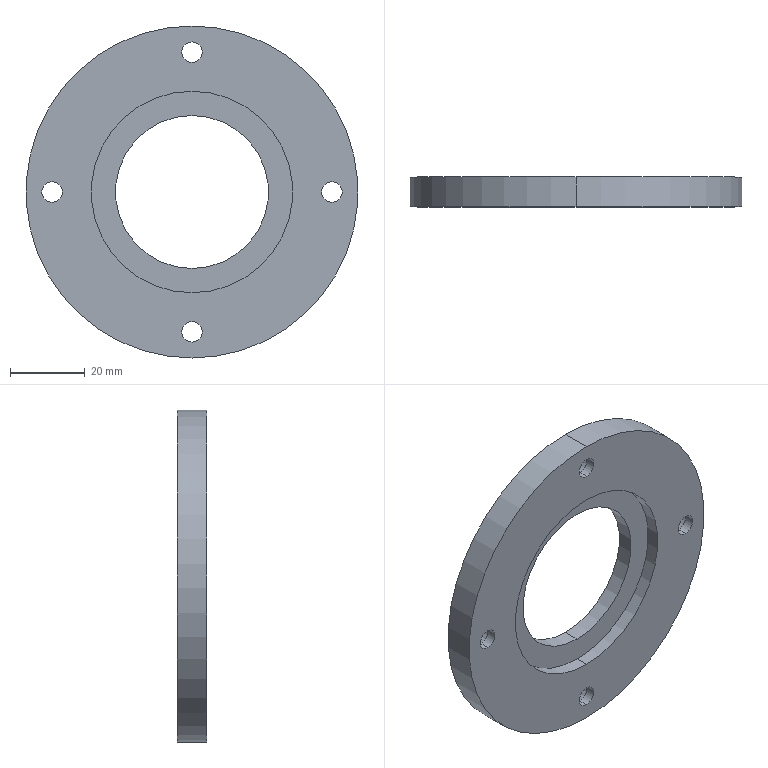Part | STEP file | 0229_220_Holder | 1 solid | 29 faces | box 89 x 8 x 89 mm | volume 33937 mm3 | cylinder 22 | plane 7 | commonest cylinder face diameters 5.5 x8 9.5 x8 41 x2 54 x2 89 x2